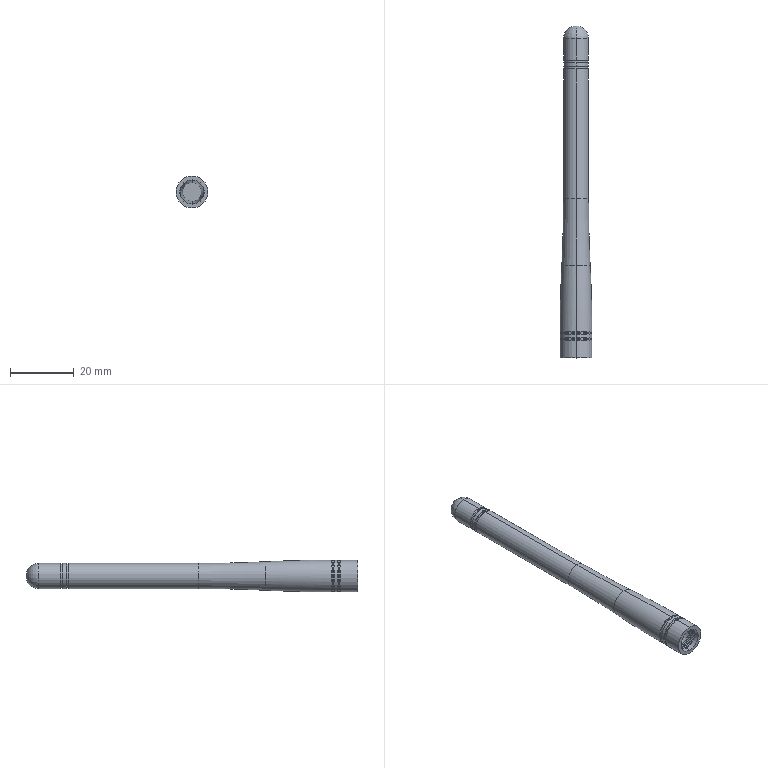Part | SolidWorks | features Fillet 1, Revolution 1 | 1 solid | 92 faces | box 10 x 104.2 x 10 mm | volume 2546 mm3 | torus 42 | cylinder 34 | plane 16 | commonest cylinder face diameters 7.6 x8 7.9 x6 8 x6 7.5 x4 9.6 x4 10 x4